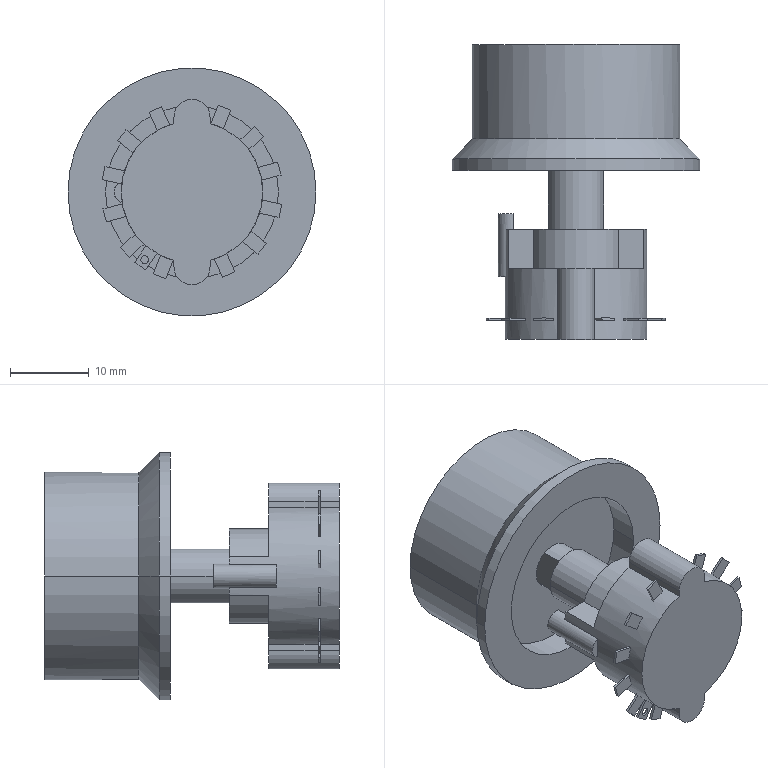Part | NX | 1 solid | 113 faces | box 31.547 x 37.5 x 31.547 mm | volume 11606 mm3 | plane 89 | cylinder 22 | cone 2 | commonest cylinder face diameters 6 x3 18 x3 1 x2 4.6 x2 7 x2 12 x2